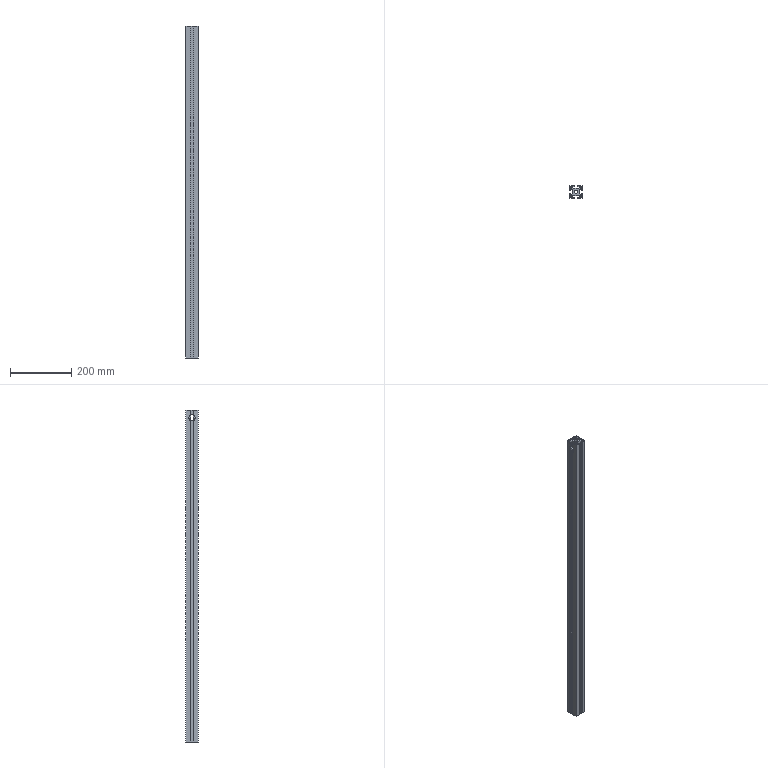Part | SolidWorks | features BaseBody 1 | 1 solid | 82 faces | box 40 x 40 x 1080 mm | volume 854909 mm3 | plane 68 | cylinder 14 | commonest cylinder face diameters 6 x8 20.5 x4 10.5 x2